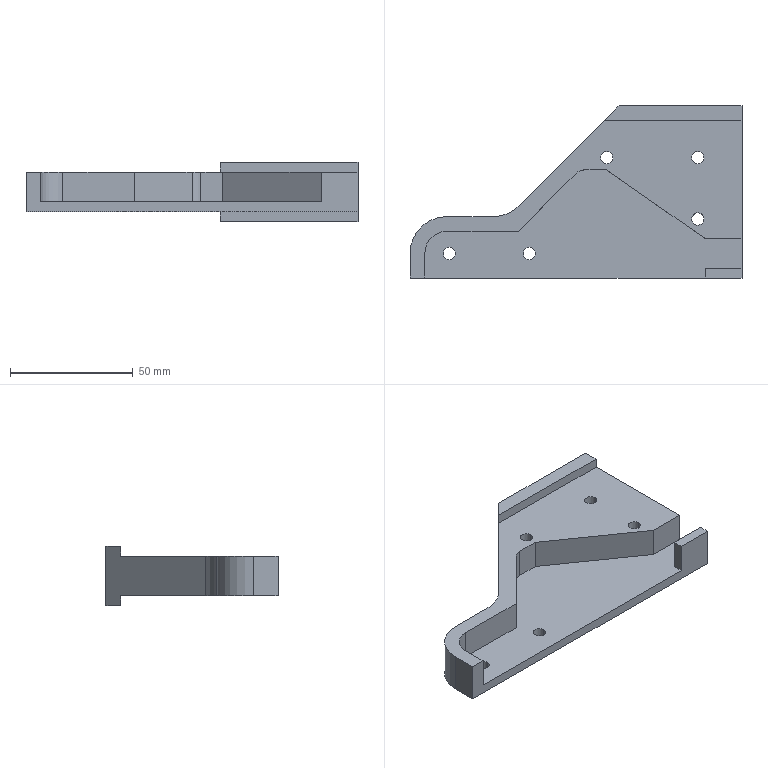Part | STEP file | Ngam kep 1 | 1 solid | 40 faces | box 135 x 70 x 24 mm | volume 65929 mm3 | plane 22 | cylinder 16 | cone 2 | commonest cylinder face diameters 5 x10 6.8 x2 30 x2 10 x1 18 x1